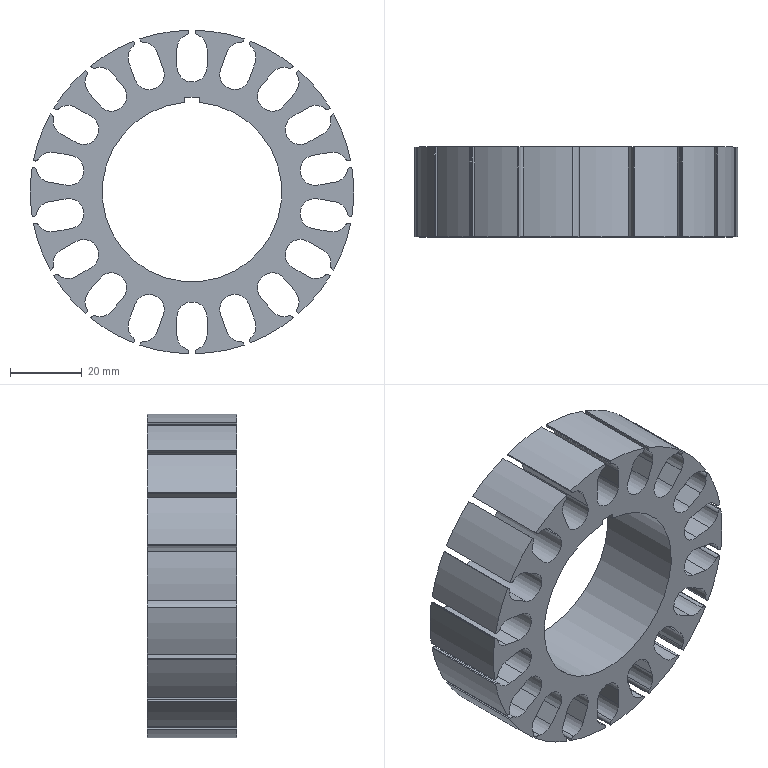Part | NX | features BREP 1 | 1 solid | 186 faces | box 90 x 25 x 89.982 mm | volume 65029 mm3 | plane 77 | cylinder 73 | spline 36 | commonest cylinder face diameters 8.4 x54 90 x18 50 x1